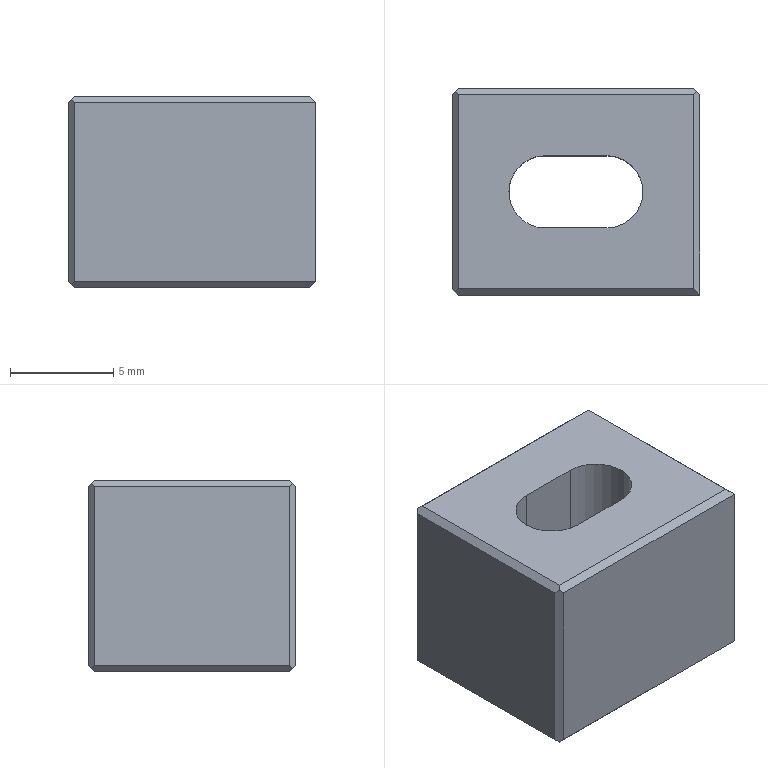Part | NX | 1 solid | 22 faces | box 12 x 10 x 9.3 mm | volume 923.798 mm3 | plane 19 | cylinder 3 | commonest cylinder face diameters 3.5 x3
STEP:
#1=CARTESIAN_POINT('',(-158.2,155.,-51.9));
#2=VERTEX_POINT('',#1);
#3=CARTESIAN_POINT('',(-146.5,155.,-51.9));
#4=VERTEX_POINT('',#3);
#5=CARTESIAN_POINT('',(-152.35,155.,-51.9));
#6=DIRECTION('',(1.,0.,0.));
#7=VECTOR('',#6,1000.);
#8=LINE('',#5,#7);
#9=EDGE_CURVE('',#2,#4,#8,.T.);
#10=ORIENTED_EDGE('',*,*,#9,.T.);
#11=CARTESIAN_POINT('',(-146.5,155.,-43.2));
#12=VERTEX_POINT('',#11);
#13=CARTESIAN_POINT('',(-146.5,155.,-50.566));
#14=DIRECTION('',(0.,0.,1.));
#15=VECTOR('',#14,1000.);
#16=LINE('',#13,#15);
#17=EDGE_CURVE('',#4,#12,#16,.T.);
#18=ORIENTED_EDGE('',*,*,#17,.T.);
#19=CARTESIAN_POINT('',(-158.2,155.,-43.2));
#20=VERTEX_POINT('',#19);
#21=CARTESIAN_POINT('',(-152.5,155.,-43.2));
#22=DIRECTION('',(1.,0.,0.));
#23=VECTOR('',#22,1000.);
#24=LINE('',#21,#23);
#25=EDGE_CURVE('',#20,#12,#24,.T.);
#26=ORIENTED_EDGE('',*,*,#25,.F.);
#27=CARTESIAN_POINT('',(-158.2,155.,-50.566));
#28=DIRECTION('',(0.,0.,1.));
#29=VECTOR('',#28,1000.);
#30=LINE('',#27,#29);
#31=EDGE_CURVE('',#2,#20,#30,.T.);
#32=ORIENTED_EDGE('',*,*,#31,.F.);
#33=EDGE_LOOP('',(#10,#18,#26,#32));
#34=FACE_BOUND('',#33,.T.);
#35=CARTESIAN_POINT('',(-163.5,155.,-58.9));
#36=DIRECTION('',(0.,-1.,0.));
#37=DIRECTION('',(0.,0.,-1.));
#38=AXIS2_PLACEMENT_3D('',#35,#36,#37);
#39=PLANE('',#38);
#40=ADVANCED_FACE('',(#34),#39,.T.);
#41=CARTESIAN_POINT('',(-146.8,164.7,-52.2));
#42=VERTEX_POINT('',#41);
#43=CARTESIAN_POINT('',(-158.2,164.7,-52.2));
#44=VERTEX_POINT('',#43);
#45=CARTESIAN_POINT('',(-152.5,164.7,-52.2));
#46=DIRECTION('',(-1.,0.,0.));
#47=VECTOR('',#46,1000.);
#48=LINE('',#45,#47);
#49=EDGE_CURVE('',#42,#44,#48,.T.);
#50=ORIENTED_EDGE('',*,*,#49,.F.);
#51=CARTESIAN_POINT('',(-146.8,155.3,-52.2));
#52=VERTEX_POINT('',#51);
#53=CARTESIAN_POINT('',(-146.8,159.85,-52.2));
#54=DIRECTION('',(0.,-1.,0.));
#55=VECTOR('',#54,1000.);
#56=LINE('',#53,#55);
#57=EDGE_CURVE('',#42,#52,#56,.T.);
#58=ORIENTED_EDGE('',*,*,#57,.T.);
#59=CARTESIAN_POINT('',(-158.2,155.3,-52.2));
#60=VERTEX_POINT('',#59);
#61=CARTESIAN_POINT('',(-152.35,155.3,-52.2));
#62=DIRECTION('',(1.,0.,0.));
#63=VECTOR('',#62,1000.);
#64=LINE('',#61,#63);
#65=EDGE_CURVE('',#60,#52,#64,.T.);
#66=ORIENTED_EDGE('',*,*,#65,.F.);
#67=CARTESIAN_POINT('',(-158.2,160.,-52.2));
#68=DIRECTION('',(0.,-1.,0.));
#69=VECTOR('',#68,1000.);
#70=LINE('',#67,#69);
#71=EDGE_CURVE('',#44,#60,#70,.T.);
#72=ORIENTED_EDGE('',*,*,#71,.F.);
#73=EDGE_LOOP('',(#50,#58,#66,#72));
#74=FACE_BOUND('',#73,.T.);
#75=CARTESIAN_POINT('',(-154.,158.25,-52.2));
#76=VERTEX_POINT('',#75);
#77=CARTESIAN_POINT('',(-151.,158.25,-52.2));
#78=VERTEX_POINT('',#77);
#79=CARTESIAN_POINT('',(-163.5,158.25,-52.2));
#80=DIRECTION('',(1.,0.,0.));
#81=VECTOR('',#80,1000.);
#82=LINE('',#79,#81);
#83=EDGE_CURVE('',#76,#78,#82,.T.);
#84=ORIENTED_EDGE('',*,*,#83,.T.);
#85=CARTESIAN_POINT('',(-151.,161.75,-52.2));
#86=VERTEX_POINT('',#85);
#87=CARTESIAN_POINT('',(-151.,160.,-52.2));
#88=DIRECTION('',(0.,0.,-1.));
#89=DIRECTION('',(-1.,0.,0.));
#90=AXIS2_PLACEMENT_3D('',#87,#88,#89);
#91=CIRCLE('',#90,1.75);
#92=EDGE_CURVE('',#86,#78,#91,.T.);
#93=ORIENTED_EDGE('',*,*,#92,.F.);
#94=CARTESIAN_POINT('',(-154.,161.75,-52.2));
#95=VERTEX_POINT('',#94);
#96=CARTESIAN_POINT('',(-163.5,161.75,-52.2));
#97=DIRECTION('',(-1.,0.,0.));
#98=VECTOR('',#97,1000.);
#99=LINE('',#96,#98);
#100=EDGE_CURVE('',#86,#95,#99,.T.);
#101=ORIENTED_EDGE('',*,*,#100,.T.);
#102=CARTESIAN_POINT('',(-155.75,160.,-52.2));
#103=VERTEX_POINT('',#102);
#104=CARTESIAN_POINT('',(-154.,160.,-52.2));
#105=DIRECTION('',(0.,0.,-1.));
#106=DIRECTION('',(-1.,0.,0.));
#107=AXIS2_PLACEMENT_3D('',#104,#105,#106);
#108=CIRCLE('',#107,1.75);
#109=EDGE_CURVE('',#103,#95,#108,.T.);
#110=ORIENTED_EDGE('',*,*,#109,.F.);
#111=CARTESIAN_POINT('',(-154.,160.,-52.2));
#112=DIRECTION('',(0.,0.,-1.));
#113=DIRECTION('',(-1.,0.,0.));
#114=AXIS2_PLACEMENT_3D('',#111,#112,#113);
#115=CIRCLE('',#114,1.75);
#116=EDGE_CURVE('',#76,#103,#115,.T.);
#117=ORIENTED_EDGE('',*,*,#116,.F.);
#118=EDGE_LOOP('',(#84,#93,#101,#110,#117));
#119=FACE_BOUND('',#118,.T.);
#120=CARTESIAN_POINT('',(-163.5,162.,-52.2));
#121=DIRECTION('',(0.,0.,-1.));
#122=DIRECTION('',(0.,-1.,0.));
#123=AXIS2_PLACEMENT_3D('',#120,#121,#122);
#124=PLANE('',#123);
#125=ADVANCED_FACE('',(#74,#119),#124,.T.);
#126=CARTESIAN_POINT('',(-146.8,165.,-51.9));
#127=VERTEX_POINT('',#126);
#128=CARTESIAN_POINT('',(-158.2,165.,-51.9));
#129=VERTEX_POINT('',#128);
#130=CARTESIAN_POINT('',(-152.5,165.,-51.9));
#131=DIRECTION('',(-1.,0.,0.));
#132=VECTOR('',#131,1000.);
#133=LINE('',#130,#132);
#134=EDGE_CURVE('',#127,#129,#133,.T.);
#135=ORIENTED_EDGE('',*,*,#134,.T.);
#136=CARTESIAN_POINT('',(-158.2,165.,-43.2));
#137=VERTEX_POINT('',#136);
#138=CARTESIAN_POINT('',(-158.2,165.,-50.566));
#139=DIRECTION('',(0.,0.,-1.));
#140=VECTOR('',#139,1000.);
#141=LINE('',#138,#140);
#142=EDGE_CURVE('',#137,#129,#141,.T.);
#143=ORIENTED_EDGE('',*,*,#142,.F.);
#144=CARTESIAN_POINT('',(-146.8,165.,-43.2));
#145=VERTEX_POINT('',#144);
#146=CARTESIAN_POINT('',(-152.5,165.,-43.2));
#147=DIRECTION('',(-1.,0.,0.));
#148=VECTOR('',#147,1000.);
#149=LINE('',#146,#148);
#150=EDGE_CURVE('',#145,#137,#149,.T.);
#151=ORIENTED_EDGE('',*,*,#150,.F.);
#152=CARTESIAN_POINT('',(-146.8,165.,-50.566));
#153=DIRECTION('',(0.,0.,-1.));
#154=VECTOR('',#153,1000.);
#155=LINE('',#152,#154);
#156=EDGE_CURVE('',#145,#127,#155,.T.);
#157=ORIENTED_EDGE('',*,*,#156,.T.);
#158=EDGE_LOOP('',(#135,#143,#151,#157));
#159=FACE_BOUND('',#158,.T.);
#160=CARTESIAN_POINT('',(-163.5,165.,-42.9));
#161=DIRECTION('',(0.,1.,0.));
#162=DIRECTION('',(1.,0.,0.));
#163=AXIS2_PLACEMENT_3D('',#160,#161,#162);
#164=PLANE('',#163);
#165=ADVANCED_FACE('',(#159),#164,.T.);
#166=CARTESIAN_POINT('',(-158.2,155.3,-42.9));
#167=VERTEX_POINT('',#166);
#168=CARTESIAN_POINT('',(-158.2,164.7,-42.9));
#169=VERTEX_POINT('',#168);
#170=CARTESIAN_POINT('',(-158.2,160.,-42.9));
#171=DIRECTION('',(0.,1.,0.));
#172=VECTOR('',#171,1000.);
#173=LINE('',#170,#172);
#174=EDGE_CURVE('',#167,#169,#173,.T.);
#175=ORIENTED_EDGE('',*,*,#174,.F.);
#176=CARTESIAN_POINT('',(-146.8,155.3,-42.9));
#177=VERTEX_POINT('',#176);
#178=CARTESIAN_POINT('',(-152.5,155.3,-42.9));
#179=DIRECTION('',(1.,0.,0.));
#180=VECTOR('',#179,1000.);
#181=LINE('',#178,#180);
#182=EDGE_CURVE('',#167,#177,#181,.T.);
#183=ORIENTED_EDGE('',*,*,#182,.T.);
#184=CARTESIAN_POINT('',(-146.8,164.7,-42.9));
#185=VERTEX_POINT('',#184);
#186=CARTESIAN_POINT('',(-146.8,160.,-42.9));
#187=DIRECTION('',(0.,1.,0.));
#188=VECTOR('',#187,1000.);
#189=LINE('',#186,#188);
#190=EDGE_CURVE('',#177,#185,#189,.T.);
#191=ORIENTED_EDGE('',*,*,#190,.T.);
#192=CARTESIAN_POINT('',(-152.5,164.7,-42.9));
#193=DIRECTION('',(-1.,0.,0.));
#194=VECTOR('',#193,1000.);
#195=LINE('',#192,#194);
#196=EDGE_CURVE('',#185,#169,#195,.T.);
#197=ORIENTED_EDGE('',*,*,#196,.T.);
#198=EDGE_LOOP('',(#175,#183,#191,#197));
#199=FACE_BOUND('',#198,.T.);
#200=CARTESIAN_POINT('',(-151.,161.75,-42.9));
#201=VERTEX_POINT('',#200);
#202=CARTESIAN_POINT('',(-154.,161.75,-42.9));
#203=VERTEX_POINT('',#202);
#204=CARTESIAN_POINT('',(-163.5,161.75,-42.9));
#205=DIRECTION('',(-1.,0.,0.));
#206=VECTOR('',#205,1000.);
#207=LINE('',#204,#206);
#208=EDGE_CURVE('',#201,#203,#207,.T.);
#209=ORIENTED_EDGE('',*,*,#208,.F.);
#210=CARTESIAN_POINT('',(-151.,158.25,-42.9));
#211=VERTEX_POINT('',#210);
#212=CARTESIAN_POINT('',(-151.,160.,-42.9));
#213=DIRECTION('',(0.,0.,-1.));
#214=DIRECTION('',(-1.,0.,0.));
#215=AXIS2_PLACEMENT_3D('',#212,#213,#214);
#216=CIRCLE('',#215,1.75);
#217=EDGE_CURVE('',#201,#211,#216,.T.);
#218=ORIENTED_EDGE('',*,*,#217,.T.);
#219=CARTESIAN_POINT('',(-154.,158.25,-42.9));
#220=VERTEX_POINT('',#219);
#221=CARTESIAN_POINT('',(-163.5,158.25,-42.9));
#222=DIRECTION('',(1.,0.,0.));
#223=VECTOR('',#222,1000.);
#224=LINE('',#221,#223);
#225=EDGE_CURVE('',#220,#211,#224,.T.);
#226=ORIENTED_EDGE('',*,*,#225,.F.);
#227=CARTESIAN_POINT('',(-155.75,160.,-42.9));
#228=VERTEX_POINT('',#227);
#229=CARTESIAN_POINT('',(-154.,160.,-42.9));
#230=DIRECTION('',(0.,0.,-1.));
#231=DIRECTION('',(-1.,0.,0.));
#232=AXIS2_PLACEMENT_3D('',#229,#230,#231);
#233=CIRCLE('',#232,1.75);
#234=EDGE_CURVE('',#220,#228,#233,.T.);
#235=ORIENTED_EDGE('',*,*,#234,.T.);
#236=CARTESIAN_POINT('',(-154.,160.,-42.9));
#237=DIRECTION('',(0.,0.,-1.));
#238=DIRECTION('',(-1.,0.,0.));
#239=AXIS2_PLACEMENT_3D('',#236,#237,#238);
#240=CIRCLE('',#239,1.75);
#241=EDGE_CURVE('',#228,#203,#240,.T.);
#242=ORIENTED_EDGE('',*,*,#241,.T.);
#243=EDGE_LOOP('',(#209,#218,#226,#235,#242));
#244=FACE_BOUND('',#243,.T.);
#245=CARTESIAN_POINT('',(-163.5,155.8,-42.9));
#246=DIRECTION('',(0.,0.,1.));
#247=DIRECTION('',(1.,0.,0.));
#248=AXIS2_PLACEMENT_3D('',#245,#246,#247);
#249=PLANE('',#248);
#250=ADVANCED_FACE('',(#199,#244),#249,.T.);
#251=CARTESIAN_POINT('',(-155.75,160.,-41.77));
#252=DIRECTION('',(0.,0.,-1.));
#253=VECTOR('',#252,1000.);
#254=LINE('',#251,#253);
#255=EDGE_CURVE('',#228,#103,#254,.T.);
#256=ORIENTED_EDGE('',*,*,#255,.F.);
#257=ORIENTED_EDGE('',*,*,#234,.F.);
#258=CARTESIAN_POINT('',(-154.,158.25,-41.77));
#259=DIRECTION('',(0.,0.,-1.));
#260=VECTOR('',#259,1000.);
#261=LINE('',#258,#260);
#262=EDGE_CURVE('',#220,#76,#261,.T.);
#263=ORIENTED_EDGE('',*,*,#262,.T.);
#264=ORIENTED_EDGE('',*,*,#116,.T.);
#265=EDGE_LOOP('',(#256,#257,#263,#264));
#266=FACE_BOUND('',#265,.T.);
#267=CARTESIAN_POINT('',(-154.,160.,-41.77));
#268=DIRECTION('',(0.,0.,-1.));
#269=DIRECTION('',(-1.,0.,0.));
#270=AXIS2_PLACEMENT_3D('',#267,#268,#269);
#271=CYLINDRICAL_SURFACE('',#270,1.75);
#272=ADVANCED_FACE('',(#266),#271,.F.);
#273=ORIENTED_EDGE('',*,*,#217,.F.);
#274=CARTESIAN_POINT('',(-151.,161.75,-41.77));
#275=DIRECTION('',(0.,0.,-1.));
#276=VECTOR('',#275,1000.);
#277=LINE('',#274,#276);
#278=EDGE_CURVE('',#201,#86,#277,.T.);
#279=ORIENTED_EDGE('',*,*,#278,.T.);
#280=ORIENTED_EDGE('',*,*,#92,.T.);
#281=CARTESIAN_POINT('',(-151.,158.25,-41.77));
#282=DIRECTION('',(0.,0.,-1.));
#283=VECTOR('',#282,1000.);
#284=LINE('',#281,#283);
#285=EDGE_CURVE('',#211,#78,#284,.T.);
#286=ORIENTED_EDGE('',*,*,#285,.F.);
#287=EDGE_LOOP('',(#273,#279,#280,#286));
#288=FACE_BOUND('',#287,.T.);
#289=CARTESIAN_POINT('',(-151.,160.,-41.77));
#290=DIRECTION('',(0.,0.,-1.));
#291=DIRECTION('',(-1.,0.,0.));
#292=AXIS2_PLACEMENT_3D('',#289,#290,#291);
#293=CYLINDRICAL_SURFACE('',#292,1.75);
#294=ADVANCED_FACE('',(#288),#293,.F.);
#295=ORIENTED_EDGE('',*,*,#83,.F.);
#296=ORIENTED_EDGE('',*,*,#262,.F.);
#297=ORIENTED_EDGE('',*,*,#225,.T.);
#298=ORIENTED_EDGE('',*,*,#285,.T.);
#299=EDGE_LOOP('',(#295,#296,#297,#298));
#300=FACE_BOUND('',#299,.T.);
#301=CARTESIAN_POINT('',(-154.,158.25,-41.77));
#302=DIRECTION('',(0.,-1.,0.));
#303=DIRECTION('',(0.,0.,-1.));
#304=AXIS2_PLACEMENT_3D('',#301,#302,#303);
#305=PLANE('',#304);
#306=ADVANCED_FACE('',(#300),#305,.F.);
#307=ORIENTED_EDGE('',*,*,#208,.T.);
#308=CARTESIAN_POINT('',(-154.,161.75,-41.77));
#309=DIRECTION('',(0.,0.,-1.));
#310=VECTOR('',#309,1000.);
#311=LINE('',#308,#310);
#312=EDGE_CURVE('',#203,#95,#311,.T.);
#313=ORIENTED_EDGE('',*,*,#312,.T.);
#314=ORIENTED_EDGE('',*,*,#100,.F.);
#315=ORIENTED_EDGE('',*,*,#278,.F.);
#316=EDGE_LOOP('',(#307,#313,#314,#315));
#317=FACE_BOUND('',#316,.T.);
#318=CARTESIAN_POINT('',(-151.,161.75,-41.77));
#319=DIRECTION('',(0.,1.,0.));
#320=DIRECTION('',(1.,0.,0.));
#321=AXIS2_PLACEMENT_3D('',#318,#319,#320);
#322=PLANE('',#321);
#323=ADVANCED_FACE('',(#317),#322,.F.);
#324=ORIENTED_EDGE('',*,*,#25,.T.);
#325=CARTESIAN_POINT('',(-163.5,172.,-26.2));
#326=DIRECTION('',(0.5774,-0.5774,-0.5774));
#327=VECTOR('',#326,1000.);
#328=LINE('',#325,#327);
#329=EDGE_CURVE('',#177,#12,#328,.T.);
#330=ORIENTED_EDGE('',*,*,#329,.F.);
#331=ORIENTED_EDGE('',*,*,#182,.F.);
#332=CARTESIAN_POINT('',(-158.35,155.15,-43.05));
#333=VERTEX_POINT('',#332);
#334=CARTESIAN_POINT('',(-165.866,147.634,-50.566));
#335=DIRECTION('',(0.5774,0.5774,0.5774));
#336=VECTOR('',#335,1000.);
#337=LINE('',#334,#336);
#338=EDGE_CURVE('',#333,#167,#337,.T.);
#339=ORIENTED_EDGE('',*,*,#338,.F.);
#340=CARTESIAN_POINT('',(-150.834,147.634,-50.566));
#341=DIRECTION('',(0.5774,-0.5774,-0.5774));
#342=VECTOR('',#341,1000.);
#343=LINE('',#340,#342);
#344=EDGE_CURVE('',#333,#20,#343,.T.);
#345=ORIENTED_EDGE('',*,*,#344,.T.);
#346=EDGE_LOOP('',(#324,#330,#331,#339,#345));
#347=FACE_BOUND('',#346,.T.);
#348=CARTESIAN_POINT('',(-152.5,155.15,-43.05));
#349=DIRECTION('',(0.,0.7071,-0.7071));
#350=DIRECTION('',(-1.,0.,0.));
#351=AXIS2_PLACEMENT_3D('',#348,#349,#350);
#352=PLANE('',#351);
#353=ADVANCED_FACE('',(#347),#352,.F.);
#354=ORIENTED_EDGE('',*,*,#150,.T.);
#355=CARTESIAN_POINT('',(-158.35,164.85,-43.05));
#356=VERTEX_POINT('',#355);
#357=CARTESIAN_POINT('',(-169.713,153.487,-31.687));
#358=DIRECTION('',(0.5774,0.5774,-0.5774));
#359=VECTOR('',#358,1000.);
#360=LINE('',#357,#359);
#361=EDGE_CURVE('',#356,#137,#360,.T.);
#362=ORIENTED_EDGE('',*,*,#361,.F.);
#363=CARTESIAN_POINT('',(-146.987,153.487,-31.687));
#364=DIRECTION('',(-0.5774,0.5774,-0.5774));
#365=VECTOR('',#364,1000.);
#366=LINE('',#363,#365);
#367=EDGE_CURVE('',#169,#356,#366,.T.);
#368=ORIENTED_EDGE('',*,*,#367,.F.);
#369=ORIENTED_EDGE('',*,*,#196,.F.);
#370=CARTESIAN_POINT('',(-146.65,164.85,-43.05));
#371=VERTEX_POINT('',#370);
#372=CARTESIAN_POINT('',(-163.5,148.,-26.2));
#373=DIRECTION('',(-0.5774,-0.5774,0.5774));
#374=VECTOR('',#373,1000.);
#375=LINE('',#372,#374);
#376=EDGE_CURVE('',#371,#185,#375,.T.);
#377=ORIENTED_EDGE('',*,*,#376,.F.);
#378=CARTESIAN_POINT('',(-163.5,181.7,-59.9));
#379=DIRECTION('',(0.5774,-0.5774,0.5774));
#380=VECTOR('',#379,1000.);
#381=LINE('',#378,#380);
#382=EDGE_CURVE('',#145,#371,#381,.T.);
#383=ORIENTED_EDGE('',*,*,#382,.F.);
#384=EDGE_LOOP('',(#354,#362,#368,#369,#377,#383));
#385=FACE_BOUND('',#384,.T.);
#386=CARTESIAN_POINT('',(-152.5,164.85,-43.05));
#387=DIRECTION('',(0.,-0.7071,-0.7071));
#388=DIRECTION('',(0.,-0.7071,0.7071));
#389=AXIS2_PLACEMENT_3D('',#386,#387,#388);
#390=PLANE('',#389);
#391=ADVANCED_FACE('',(#385),#390,.F.);
#392=ORIENTED_EDGE('',*,*,#49,.T.);
#393=CARTESIAN_POINT('',(-158.35,164.85,-52.05));
#394=VERTEX_POINT('',#393);
#395=CARTESIAN_POINT('',(-146.987,153.487,-63.413));
#396=DIRECTION('',(-0.5774,0.5774,0.5774));
#397=VECTOR('',#396,1000.);
#398=LINE('',#395,#397);
#399=EDGE_CURVE('',#44,#394,#398,.T.);
#400=ORIENTED_EDGE('',*,*,#399,.T.);
#401=CARTESIAN_POINT('',(-169.713,153.487,-63.413));
#402=DIRECTION('',(-0.5774,-0.5774,-0.5774));
#403=VECTOR('',#402,1000.);
#404=LINE('',#401,#403);
#405=EDGE_CURVE('',#129,#394,#404,.T.);
#406=ORIENTED_EDGE('',*,*,#405,.F.);
#407=ORIENTED_EDGE('',*,*,#134,.F.);
#408=CARTESIAN_POINT('',(-146.65,164.85,-52.05));
#409=VERTEX_POINT('',#408);
#410=CARTESIAN_POINT('',(-163.5,181.7,-35.2));
#411=DIRECTION('',(0.5774,-0.5774,-0.5774));
#412=VECTOR('',#411,1000.);
#413=LINE('',#410,#412);
#414=EDGE_CURVE('',#127,#409,#413,.T.);
#415=ORIENTED_EDGE('',*,*,#414,.T.);
#416=CARTESIAN_POINT('',(-158.013,153.487,-63.413));
#417=DIRECTION('',(0.5774,0.5774,0.5774));
#418=VECTOR('',#417,1000.);
#419=LINE('',#416,#418);
#420=EDGE_CURVE('',#42,#409,#419,.T.);
#421=ORIENTED_EDGE('',*,*,#420,.F.);
#422=EDGE_LOOP('',(#392,#400,#406,#407,#415,#421));
#423=FACE_BOUND('',#422,.T.);
#424=CARTESIAN_POINT('',(-152.5,164.85,-52.05));
#425=DIRECTION('',(0.,-0.7071,0.7071));
#426=DIRECTION('',(-1.,0.,0.));
#427=AXIS2_PLACEMENT_3D('',#424,#425,#426);
#428=PLANE('',#427);
#429=ADVANCED_FACE('',(#423),#428,.F.);
#430=ORIENTED_EDGE('',*,*,#9,.F.);
#431=CARTESIAN_POINT('',(-158.35,155.15,-52.05));
#432=VERTEX_POINT('',#431);
#433=CARTESIAN_POINT('',(-156.866,153.666,-50.566));
#434=DIRECTION('',(-0.5774,0.5774,-0.5774));
#435=VECTOR('',#434,1000.);
#436=LINE('',#433,#435);
#437=EDGE_CURVE('',#2,#432,#436,.T.);
#438=ORIENTED_EDGE('',*,*,#437,.T.);
#439=CARTESIAN_POINT('',(-159.834,153.666,-50.566));
#440=DIRECTION('',(0.5774,0.5774,-0.5774));
#441=VECTOR('',#440,1000.);
#442=LINE('',#439,#441);
#443=EDGE_CURVE('',#432,#60,#442,.T.);
#444=ORIENTED_EDGE('',*,*,#443,.T.);
#445=ORIENTED_EDGE('',*,*,#65,.T.);
#446=CARTESIAN_POINT('',(-163.5,172.,-68.9));
#447=DIRECTION('',(-0.5774,0.5774,-0.5774));
#448=VECTOR('',#447,1000.);
#449=LINE('',#446,#448);
#450=EDGE_CURVE('',#4,#52,#449,.T.);
#451=ORIENTED_EDGE('',*,*,#450,.F.);
#452=EDGE_LOOP('',(#430,#438,#444,#445,#451));
#453=FACE_BOUND('',#452,.T.);
#454=CARTESIAN_POINT('',(-152.35,155.15,-52.05));
#455=DIRECTION('',(0.,-0.7071,-0.7071));
#456=DIRECTION('',(0.,-0.7071,0.7071));
#457=AXIS2_PLACEMENT_3D('',#454,#455,#456);
#458=PLANE('',#457);
#459=ADVANCED_FACE('',(#453),#458,.T.);
#460=CARTESIAN_POINT('',(-146.5,164.7,-51.9));
#461=VERTEX_POINT('',#460);
#462=CARTESIAN_POINT('',(-146.5,159.85,-51.9));
#463=DIRECTION('',(0.,-1.,0.));
#464=VECTOR('',#463,1000.);
#465=LINE('',#462,#464);
#466=EDGE_CURVE('',#461,#4,#465,.T.);
#467=ORIENTED_EDGE('',*,*,#466,.F.);
#468=CARTESIAN_POINT('',(-146.5,164.7,-43.2));
#469=VERTEX_POINT('',#468);
#470=CARTESIAN_POINT('',(-146.5,164.7,-50.566));
#471=DIRECTION('',(0.,0.,-1.));
#472=VECTOR('',#471,1000.);
#473=LINE('',#470,#472);
#474=EDGE_CURVE('',#469,#461,#473,.T.);
#475=ORIENTED_EDGE('',*,*,#474,.F.);
#476=CARTESIAN_POINT('',(-146.5,160.,-43.2));
#477=DIRECTION('',(0.,1.,0.));
#478=VECTOR('',#477,1000.);
#479=LINE('',#476,#478);
#480=EDGE_CURVE('',#12,#469,#479,.T.);
#481=ORIENTED_EDGE('',*,*,#480,.F.);
#482=ORIENTED_EDGE('',*,*,#17,.F.);
#483=EDGE_LOOP('',(#467,#475,#481,#482));
#484=FACE_BOUND('',#483,.T.);
#485=CARTESIAN_POINT('',(-146.5,153.487,-50.566));
#486=DIRECTION('',(-1.,0.,0.));
#487=DIRECTION('',(0.,0.,1.));
#488=AXIS2_PLACEMENT_3D('',#485,#486,#487);
#489=PLANE('',#488);
#490=ADVANCED_FACE('',(#484),#489,.F.);
#491=ORIENTED_EDGE('',*,*,#474,.T.);
#492=CARTESIAN_POINT('',(-163.5,181.7,-68.9));
#493=DIRECTION('',(0.5774,-0.5774,0.5774));
#494=VECTOR('',#493,1000.);
#495=LINE('',#492,#494);
#496=EDGE_CURVE('',#409,#461,#495,.T.);
#497=ORIENTED_EDGE('',*,*,#496,.F.);
#498=ORIENTED_EDGE('',*,*,#414,.F.);
#499=ORIENTED_EDGE('',*,*,#156,.F.);
#500=ORIENTED_EDGE('',*,*,#382,.T.);
#501=CARTESIAN_POINT('',(-163.5,181.7,-26.2));
#502=DIRECTION('',(0.5774,-0.5774,-0.5774));
#503=VECTOR('',#502,1000.);
#504=LINE('',#501,#503);
#505=EDGE_CURVE('',#371,#469,#504,.T.);
#506=ORIENTED_EDGE('',*,*,#505,.T.);
#507=EDGE_LOOP('',(#491,#497,#498,#499,#500,#506));
#508=FACE_BOUND('',#507,.T.);
#509=CARTESIAN_POINT('',(-146.65,164.85,-48.55));
#510=DIRECTION('',(-0.7071,-0.7071,0.));
#511=DIRECTION('',(-0.7071,0.7071,0.));
#512=AXIS2_PLACEMENT_3D('',#509,#510,#511);
#513=PLANE('',#512);
#514=ADVANCED_FACE('',(#508),#513,.F.);
#515=ORIENTED_EDGE('',*,*,#480,.T.);
#516=ORIENTED_EDGE('',*,*,#505,.F.);
#517=ORIENTED_EDGE('',*,*,#376,.T.);
#518=ORIENTED_EDGE('',*,*,#190,.F.);
#519=ORIENTED_EDGE('',*,*,#329,.T.);
#520=EDGE_LOOP('',(#515,#516,#517,#518,#519));
#521=FACE_BOUND('',#520,.T.);
#522=CARTESIAN_POINT('',(-146.65,160.,-43.05));
#523=DIRECTION('',(-0.7071,0.,-0.7071));
#524=DIRECTION('',(-0.7071,0.,0.7071));
#525=AXIS2_PLACEMENT_3D('',#522,#523,#524);
#526=PLANE('',#525);
#527=ADVANCED_FACE('',(#521),#526,.F.);
#528=ORIENTED_EDGE('',*,*,#466,.T.);
#529=ORIENTED_EDGE('',*,*,#450,.T.);
#530=ORIENTED_EDGE('',*,*,#57,.F.);
#531=ORIENTED_EDGE('',*,*,#420,.T.);
#532=ORIENTED_EDGE('',*,*,#496,.T.);
#533=EDGE_LOOP('',(#528,#529,#530,#531,#532));
#534=FACE_BOUND('',#533,.T.);
#535=CARTESIAN_POINT('',(-146.65,159.85,-52.05));
#536=DIRECTION('',(-0.7071,0.,0.7071));
#537=DIRECTION('',(0.,1.,0.));
#538=AXIS2_PLACEMENT_3D('',#535,#536,#537);
#539=PLANE('',#538);
#540=ADVANCED_FACE('',(#534),#539,.F.);
#541=CARTESIAN_POINT('',(-158.5,164.7,-51.9));
#542=VERTEX_POINT('',#541);
#543=CARTESIAN_POINT('',(-158.5,155.3,-51.9));
#544=VERTEX_POINT('',#543);
#545=CARTESIAN_POINT('',(-158.5,160.,-51.9));
#546=DIRECTION('',(0.,-1.,0.));
#547=VECTOR('',#546,1000.);
#548=LINE('',#545,#547);
#549=EDGE_CURVE('',#542,#544,#548,.T.);
#550=ORIENTED_EDGE('',*,*,#549,.T.);
#551=CARTESIAN_POINT('',(-158.5,155.3,-43.2));
#552=VERTEX_POINT('',#551);
#553=CARTESIAN_POINT('',(-158.5,155.3,-50.566));
#554=DIRECTION('',(0.,0.,1.));
#555=VECTOR('',#554,1000.);
#556=LINE('',#553,#555);
#557=EDGE_CURVE('',#544,#552,#556,.T.);
#558=ORIENTED_EDGE('',*,*,#557,.T.);
#559=CARTESIAN_POINT('',(-158.5,164.7,-43.2));
#560=VERTEX_POINT('',#559);
#561=CARTESIAN_POINT('',(-158.5,160.,-43.2));
#562=DIRECTION('',(0.,1.,0.));
#563=VECTOR('',#562,1000.);
#564=LINE('',#561,#563);
#565=EDGE_CURVE('',#552,#560,#564,.T.);
#566=ORIENTED_EDGE('',*,*,#565,.T.);
#567=CARTESIAN_POINT('',(-158.5,164.7,-50.566));
#568=DIRECTION('',(0.,0.,-1.));
#569=VECTOR('',#568,1000.);
#570=LINE('',#567,#569);
#571=EDGE_CURVE('',#560,#542,#570,.T.);
#572=ORIENTED_EDGE('',*,*,#571,.T.);
#573=EDGE_LOOP('',(#550,#558,#566,#572));
#574=FACE_BOUND('',#573,.T.);
#575=CARTESIAN_POINT('',(-158.5,153.487,-50.566));
#576=DIRECTION('',(-1.,0.,0.));
#577=DIRECTION('',(0.,0.,1.));
#578=AXIS2_PLACEMENT_3D('',#575,#576,#577);
#579=PLANE('',#578);
#580=ADVANCED_FACE('',(#574),#579,.T.);
#581=ORIENTED_EDGE('',*,*,#142,.T.);
#582=ORIENTED_EDGE('',*,*,#405,.T.);
#583=CARTESIAN_POINT('',(-169.713,153.487,-40.687));
#584=DIRECTION('',(0.5774,0.5774,-0.5774));
#585=VECTOR('',#584,1000.);
#586=LINE('',#583,#585);
#587=EDGE_CURVE('',#542,#394,#586,.T.);
#588=ORIENTED_EDGE('',*,*,#587,.F.);
#589=ORIENTED_EDGE('',*,*,#571,.F.);
#590=CARTESIAN_POINT('',(-169.713,153.487,-54.413));
#591=DIRECTION('',(0.5774,0.5774,0.5774));
#592=VECTOR('',#591,1000.);
#593=LINE('',#590,#592);
#594=EDGE_CURVE('',#560,#356,#593,.T.);
#595=ORIENTED_EDGE('',*,*,#594,.T.);
#596=ORIENTED_EDGE('',*,*,#361,.T.);
#597=EDGE_LOOP('',(#581,#582,#588,#589,#595,#596));
#598=FACE_BOUND('',#597,.T.);
#599=CARTESIAN_POINT('',(-158.35,164.85,-48.55));
#600=DIRECTION('',(-0.7071,0.7071,0.));
#601=DIRECTION('',(0.,0.,1.));
#602=AXIS2_PLACEMENT_3D('',#599,#600,#601);
#603=PLANE('',#602);
#604=ADVANCED_FACE('',(#598),#603,.T.);
#605=ORIENTED_EDGE('',*,*,#557,.F.);
#606=CARTESIAN_POINT('',(-159.834,156.634,-50.566));
#607=DIRECTION('',(-0.5774,0.5774,0.5774));
#608=VECTOR('',#607,1000.);
#609=LINE('',#606,#608);
#610=EDGE_CURVE('',#432,#544,#609,.T.);
#611=ORIENTED_EDGE('',*,*,#610,.F.);
#612=ORIENTED_EDGE('',*,*,#437,.F.);
#613=ORIENTED_EDGE('',*,*,#31,.T.);
#614=ORIENTED_EDGE('',*,*,#344,.F.);
#615=CARTESIAN_POINT('',(-156.687,153.487,-41.387));
#616=DIRECTION('',(-0.5774,0.5774,-0.5774));
#617=VECTOR('',#616,1000.);
#618=LINE('',#615,#617);
#619=EDGE_CURVE('',#333,#552,#618,.T.);
#620=ORIENTED_EDGE('',*,*,#619,.T.);
#621=EDGE_LOOP('',(#605,#611,#612,#613,#614,#620));
#622=FACE_BOUND('',#621,.T.);
#623=CARTESIAN_POINT('',(-158.35,155.15,-48.55));
#624=DIRECTION('',(-0.7071,-0.7071,0.));
#625=DIRECTION('',(-0.7071,0.7071,0.));
#626=AXIS2_PLACEMENT_3D('',#623,#624,#625);
#627=PLANE('',#626);
#628=ADVANCED_FACE('',(#622),#627,.T.);
#629=ORIENTED_EDGE('',*,*,#565,.F.);
#630=ORIENTED_EDGE('',*,*,#619,.F.);
#631=ORIENTED_EDGE('',*,*,#338,.T.);
#632=ORIENTED_EDGE('',*,*,#174,.T.);
#633=ORIENTED_EDGE('',*,*,#367,.T.);
#634=ORIENTED_EDGE('',*,*,#594,.F.);
#635=EDGE_LOOP('',(#629,#630,#631,#632,#633,#634));
#636=FACE_BOUND('',#635,.T.);
#637=CARTESIAN_POINT('',(-158.35,160.,-43.05));
#638=DIRECTION('',(-0.7071,0.,0.7071));
#639=DIRECTION('',(0.,1.,0.));
#640=AXIS2_PLACEMENT_3D('',#637,#638,#639);
#641=PLANE('',#640);
#642=ADVANCED_FACE('',(#636),#641,.T.);
#643=ORIENTED_EDGE('',*,*,#549,.F.);
#644=ORIENTED_EDGE('',*,*,#587,.T.);
#645=ORIENTED_EDGE('',*,*,#399,.F.);
#646=ORIENTED_EDGE('',*,*,#71,.T.);
#647=ORIENTED_EDGE('',*,*,#443,.F.);
#648=ORIENTED_EDGE('',*,*,#610,.T.);
#649=EDGE_LOOP('',(#643,#644,#645,#646,#647,#648));
#650=FACE_BOUND('',#649,.T.);
#651=CARTESIAN_POINT('',(-158.35,160.,-52.05));
#652=DIRECTION('',(-0.7071,0.,-0.7071));
#653=DIRECTION('',(-0.7071,0.,0.7071));
#654=AXIS2_PLACEMENT_3D('',#651,#652,#653);
#655=PLANE('',#654);
#656=ADVANCED_FACE('',(#650),#655,.T.);
#657=ORIENTED_EDGE('',*,*,#241,.F.);
#658=ORIENTED_EDGE('',*,*,#255,.T.);
#659=ORIENTED_EDGE('',*,*,#109,.T.);
#660=ORIENTED_EDGE('',*,*,#312,.F.);
#661=EDGE_LOOP('',(#657,#658,#659,#660));
#662=FACE_BOUND('',#661,.T.);
#663=CARTESIAN_POINT('',(-154.,160.,-41.77));
#664=DIRECTION('',(0.,0.,-1.));
#665=DIRECTION('',(-1.,0.,0.));
#666=AXIS2_PLACEMENT_3D('',#663,#664,#665);
#667=CYLINDRICAL_SURFACE('',#666,1.75);
#668=ADVANCED_FACE('',(#662),#667,.F.);
#669=CLOSED_SHELL('',(#40,#125,#165,#250,#272,#294,#306,#323,#353,#391,#429,#459,#490,#514,#527,#540,#580,#604,#628,#642,#656,#668));
#670=MANIFOLD_SOLID_BREP('',#669);
#671=(LENGTH_UNIT()NAMED_UNIT(*)SI_UNIT(.MILLI.,.METRE.));
#672=UNCERTAINTY_MEASURE_WITH_UNIT(LENGTH_MEASURE(0.00001),#671,'','');
#673=(NAMED_UNIT(*)PLANE_ANGLE_UNIT()SI_UNIT($,.RADIAN.));
#674=(NAMED_UNIT(*)SI_UNIT($,.STERADIAN.)SOLID_ANGLE_UNIT());
#675=(GEOMETRIC_REPRESENTATION_CONTEXT(3)GLOBAL_UNCERTAINTY_ASSIGNED_CONTEXT((#672))GLOBAL_UNIT_ASSIGNED_CONTEXT((#671,#673,#674))REPRESENTATION_CONTEXT('',''));
#676=ADVANCED_BREP_SHAPE_REPRESENTATION('',(#670),#675);